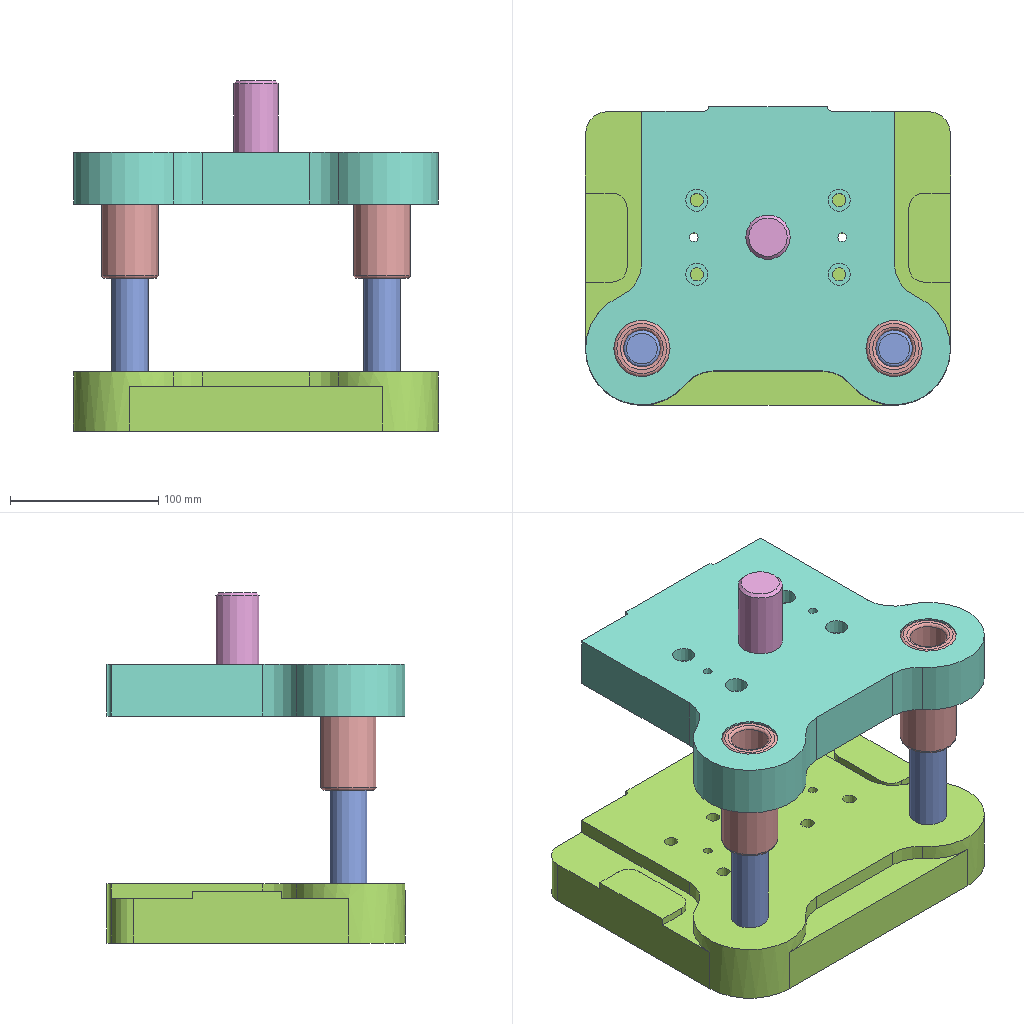Assembly | NX | 5 different items | 7 placed | box 246 x 201 x 236 mm
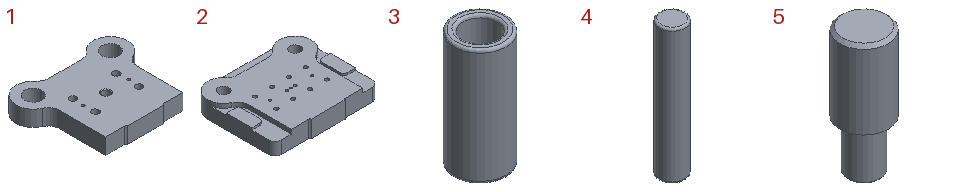Parts list (item | quantity | size | volume | features):
1 | x1 | 246 x 201 x 35 mm | 1152139 mm3 | features EXTRUDE 2, Radial Dimension 2, DATUM_CSYS 1, HOLE PACKAGE 1, SIMPLE HOLE 1, SYMBOLIC_THREAD 1
2 | x1 | 246 x 201 x 40 mm | 1748151 mm3 | features EXTRUDE 5, DATUM_CSYS 1
3 | x2 | 38 x 38 x 85 mm | 54336 mm3 | features DATUM_CSYS 2, BLEND 1, EXTRUDE 1, SKETCH 1
4 | x2 | 25 x 25 x 130 mm | 63684 mm3 | features BLEND 1, CYLINDER 1, DATUM_CSYS 1
5 | x1 | 30 x 30 x 78 mm | 43030 mm3 | features CYLINDER 3, CHAMFER 2, DATUM_CSYS 1
Mates (type | each side: item.copy, entity, surface, feature):
Concentric | 5.1 edge | 1.1 edge
Concentric | 4.1 edge | 2.1 edge | 2 times
Concentric | 3.1 edge | 1.1 edge | 2 times
Touch | 2.1 face plane Extrude(1) | assembly plane
Touch | 1.1 face plane Extrude(1) | 2.1 face plane Extrude(1)
Distance | 1.1 face plane Extrude(1) | 2.1 face plane Extrude(1)
AlignLock | 3.1 face cylinder Extrude(1) | 4.1 face cylinder Cylinder(1)